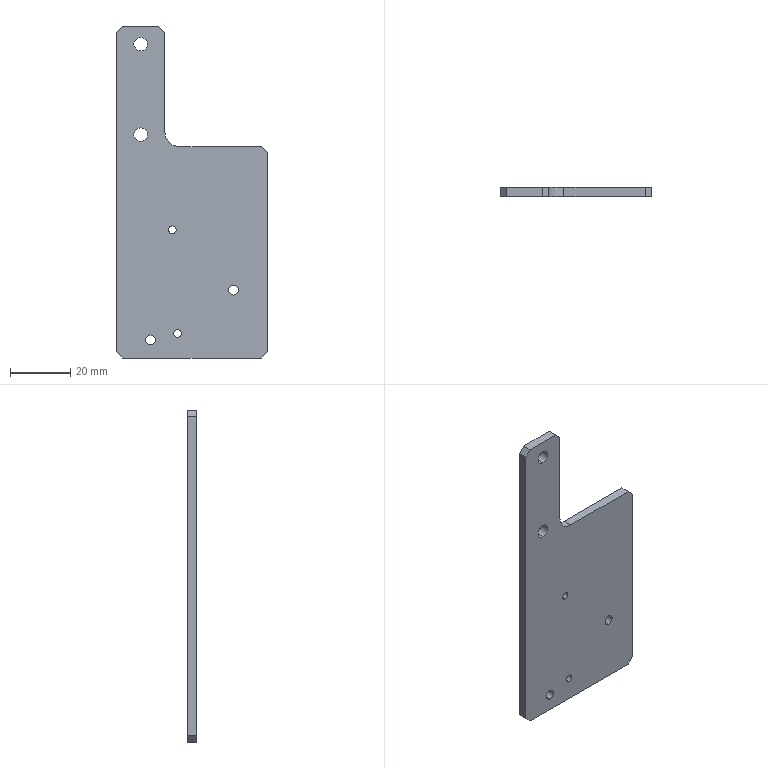Part | STEP file | vacuum generator mounting plate 2 | 1 solid | 26 faces | box 50 x 3 x 110 mm | volume 12230 mm3 | cylinder 13 | plane 13 | commonest cylinder face diameters 2.5 x4 3.3 x4 4.5 x4 10 x1